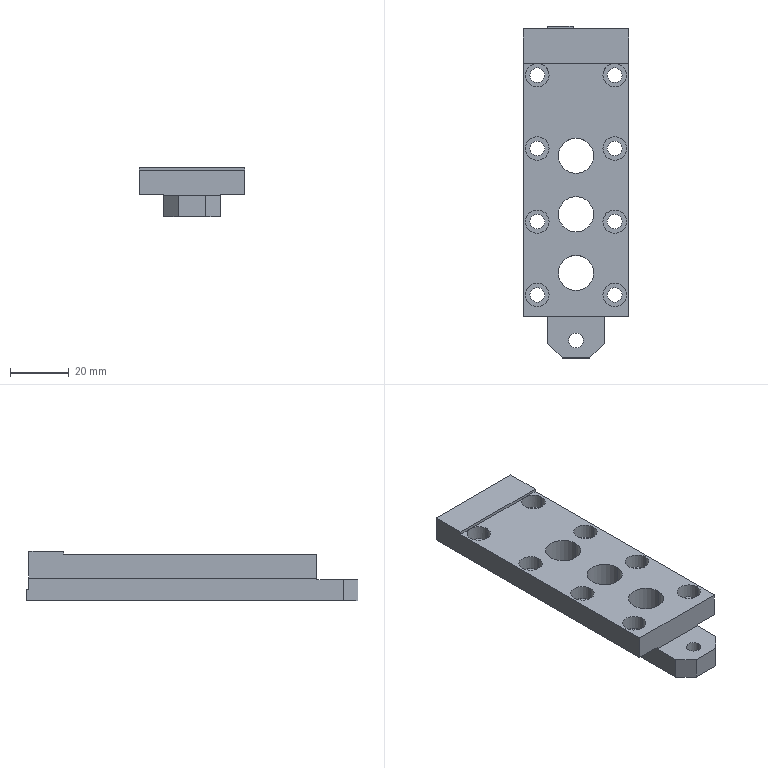Part | NX | 1 solid | 82 faces | box 36 x 113.3 x 17 mm | volume 36001 mm3 | cylinder 45 | plane 29 | cone 8 | commonest cylinder face diameters 5 x22 8 x16 12 x6 4 x1